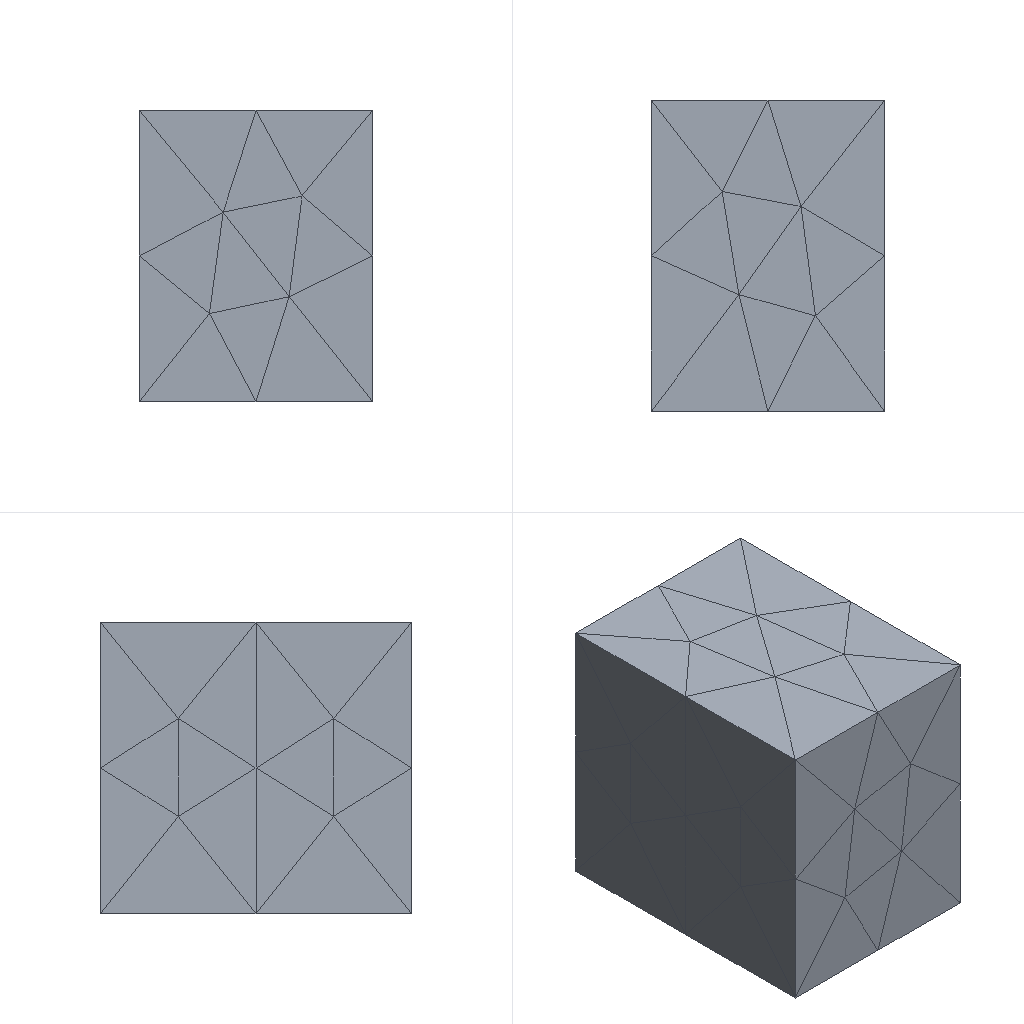Simulation study | ansys mapdl
Set-up summary:
category,name,step,type,value,unit,region
solver,ansys_mapdl
units,mm-N-s-tonne (MPa),,inferred,E=210000 density=
analysis,model,,static
mesh,nodes,,,245
mesh,elements,,,108
element_type,SOLID187,,,108
material,mat 1,,E,210000
material,mat 1,,nu,0.3
load,,model,body load temp,,,all
load,,model,force,"1000 [dir=(0, 0, -1) n=77]",,node list
bc,,model,fixed,"[dofs=UX,UY,UZ n=349]",,node list
Ansys APDL input file, long lists of numbers shortened:
/COM,ANSYS RELEASE 2026 R1           BUILD 26.1      UP20260202       09:10:33
/PREP7
/NOPR
/TITLE,2
ANTYPE, 0
*IF,_CDRDOFF,EQ,1,THEN     !if solid model was read in
_CDRDOFF=             !reset flag, numoffs already performed
*ELSE              !offset database for the following FE model
NUMOFF,NODE,      245
NUMOFF,ELEM,      108
NUMOFF,MAT ,        1
NUMOFF,TYPE,        1
*ENDIF
*SET,_RETURN ,  0.
*SET,_STATUS ,  0.
*SET,_UIQR   ,  77.
*SET,__FLOATPARAMETER__,  245.
DOF,DELETE
ETBLOCK,        1,        1
(2i9,19a9)
        1      187        0        0        0        0        0        0        0        0        0        0        0        0        0        0        0        0        0        0        0
       -1
NBLOCK,6,SOLID,       245,       245
(3i9,6e21.13e3)
        1        0        0 4.1000000000000E+001 8.0000000000000E+000
! (244 more lines like these left out)
N,UNBL,LOC,       -1,
EBLOCK,19,SOLID,       108,       108
(19i10)
         1         1         1         1         0         0         0         0        10         0         1       103         6       175       126       102       171       169       120
! (215 more lines like these left out)
        -1
MPTEMP,UNBL, 1, 1,  0.    ,
MPDATA,UNBL, 1,EX  ,       1, 1,  210000.000    ,
MPTEMP,UNBL, 1, 1,  0.    ,
MPDATA,UNBL, 1,NUXY,       1, 1, 0.3    ,
MPTEMP,UNBL, 1, 1,  0.    ,
MPDATA,UNBL, 1,PRXY,       1, 1, 0.3    ,
EXTOPT,ATTR,      0,      0,      0
EXTOPT,ESIZE,  0,  0.
EXTOPT,ACLEAR,      0
TREF,  0.
IRLF,  0
BFUNIF,TEMP,_TINY
ACEL,  0.    ,  0.    ,  0.
OMEGA,  0.    ,  0.    ,  0.
DOMEGA,  0.    ,  0.    ,  0.
CGLOC,  0.    ,  0.    ,  0.
CGOMEGA,  0.    ,  0.    ,  0.
DCGOMG,  0.    ,  0.    ,  0.
KUSE,     0
TIME,  0.
ALPHAD,  0.
BETAD,  0.
DMPRAT,  0.
DMPSTR,  0.
CRPLIM, 0.1    ,   0
CRPLIM,  0.    ,   1
NCNV,     0, 1.000000000E+12,     0,  0.    ,  0.
NEQIT,     0
ERESX,DEFA
DBLOCK,       349
(i9,a6,2(pg16.9))
        1  UX    0.00000000      0.00000000
! (348 more lines like these left out)
       -1
FBLOCK,        77
(i9,a6,2(pg16.9))
       38  FZ   -12.9870130      0.00000000
! (76 more lines like these left out)
       -1
/GO
FINISH
Results summary:
result,analysis_type_db,,,static,unstated
result,n_sets,,,1,unstated
result,load_steps[0].set,load_step=1,,1,unstated
result,load_steps[0].substep,load_step=1,,1,unstated
result,load_steps[0].time,load_step=1,,1,unstated
result,load_steps[0].freq,load_step=1,,1,unstated
result,load_steps[0].max_usum,load_step=1,,0.0004398,unstated
result,load_steps[0].max_seqv,load_step=1,,9.557,unstated
result,load_steps[0].reaction_sum.FX,load_step=1,,6.82121e-13,unstated
result,load_steps[0].reaction_sum.FY,load_step=1,,-2.1009e-11,unstated
result,load_steps[0].reaction_sum.FZ,load_step=1,,1000,unstated
result,load_steps[0].reaction_sum.MX,load_step=1,,0,unstated
result,load_steps[0].reaction_sum.MY,load_step=1,,0,unstated
result,load_steps[0].reaction_sum.MZ,load_step=1,,0,unstated
result,convergence,,,results present for all listed sets,unstated